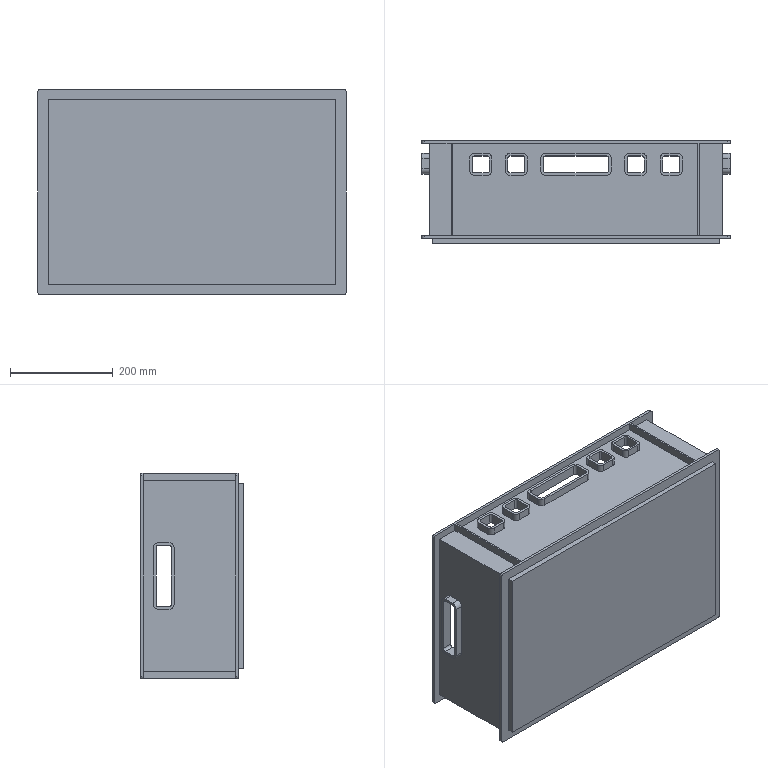Part | STEP file | Skrzynka_ver.1.1 | 2 solids | 259 faces | box 600 x 200 x 400 mm | volume 4256254 mm3 | plane 155 | cylinder 104 | commonest cylinder face diameters 8 x32 18 x32 10 x24 20 x16